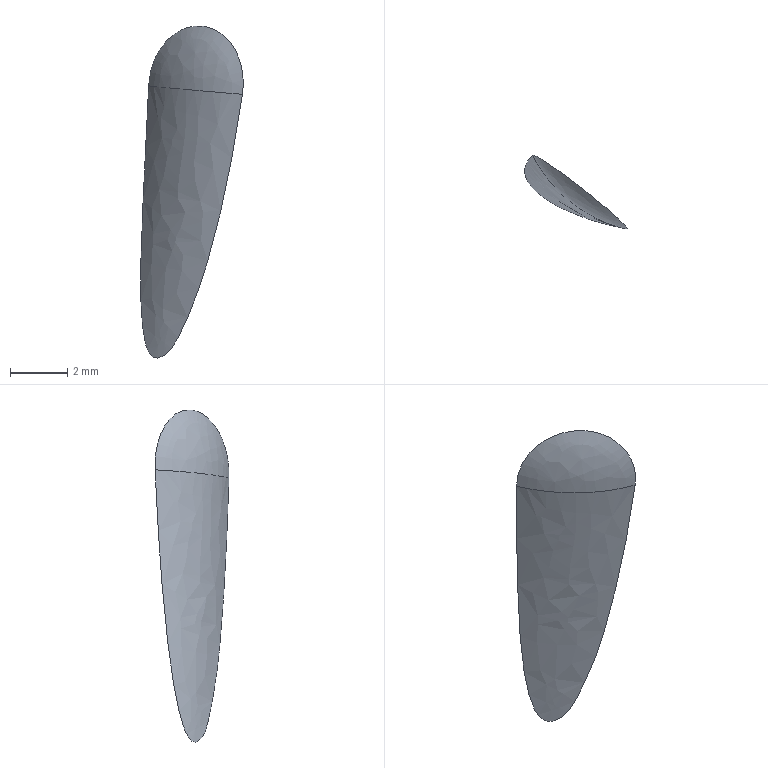Part | SolidWorks | features BaseBody 1 | 1 solid | 3 faces | box 3.595 x 2.597 x 11.647 mm | volume 8.243 mm3 | spline 3
STEP:
#1=CARTESIAN_POINT('',(82.6,89.025,-354.223));
#2=VERTEX_POINT('',#1);
#3=CARTESIAN_POINT('',(82.21,90.498,-344.695));
#4=VERTEX_POINT('',#3);
#5=CARTESIAN_POINT('',(82.6,89.025,-354.223));
#6=CARTESIAN_POINT('',(82.57,89.045,-354.233));
#7=CARTESIAN_POINT('',(82.541,89.067,-354.239));
#8=CARTESIAN_POINT('',(82.482,89.112,-354.242));
#9=CARTESIAN_POINT('',(82.452,89.136,-354.238));
#10=CARTESIAN_POINT('',(82.396,89.181,-354.222));
#11=CARTESIAN_POINT('',(82.356,89.215,-354.202));
#12=CARTESIAN_POINT('',(82.314,89.253,-354.167));
#13=CARTESIAN_POINT('',(82.294,89.272,-354.147));
#14=CARTESIAN_POINT('',(82.285,89.28,-354.137));
#15=CARTESIAN_POINT('',(82.28,89.286,-354.131));
#16=CARTESIAN_POINT('',(82.278,89.288,-354.128));
#17=CARTESIAN_POINT('',(82.246,89.319,-354.089));
#18=CARTESIAN_POINT('',(82.207,89.359,-354.027));
#19=CARTESIAN_POINT('',(82.167,89.405,-353.935));
#20=CARTESIAN_POINT('',(82.148,89.428,-353.885));
#21=CARTESIAN_POINT('',(82.14,89.437,-353.863));
#22=CARTESIAN_POINT('',(82.135,89.444,-353.848));
#23=CARTESIAN_POINT('',(82.132,89.447,-353.841));
#24=CARTESIAN_POINT('',(82.106,89.48,-353.76));
#25=CARTESIAN_POINT('',(82.085,89.51,-353.677));
#26=CARTESIAN_POINT('',(82.056,89.554,-353.538));
#27=CARTESIAN_POINT('',(82.043,89.576,-353.464));
#28=CARTESIAN_POINT('',(82.028,89.602,-353.372));
#29=CARTESIAN_POINT('',(82.021,89.615,-353.324));
#30=CARTESIAN_POINT('',(82.018,89.621,-353.303));
#31=CARTESIAN_POINT('',(82.016,89.624,-353.289));
#32=CARTESIAN_POINT('',(82.016,89.626,-353.284));
#33=CARTESIAN_POINT('',(81.977,89.702,-352.99));
#34=CARTESIAN_POINT('',(81.953,89.773,-352.649));
#35=CARTESIAN_POINT('',(81.935,89.875,-352.053));
#36=CARTESIAN_POINT('',(81.933,89.908,-351.84));
#37=CARTESIAN_POINT('',(81.933,89.957,-351.5));
#38=CARTESIAN_POINT('',(81.934,89.981,-351.325));
#39=CARTESIAN_POINT('',(81.936,90.008,-351.111));
#40=CARTESIAN_POINT('',(81.938,90.022,-351.002));
#41=CARTESIAN_POINT('',(81.939,90.029,-350.947));
#42=CARTESIAN_POINT('',(81.94,90.032,-350.919));
#43=CARTESIAN_POINT('',(81.94,90.034,-350.907));
#44=CARTESIAN_POINT('',(81.94,90.035,-350.899));
#45=CARTESIAN_POINT('',(81.94,90.035,-350.898));
#46=CARTESIAN_POINT('',(81.971,90.229,-349.305));
#47=CARTESIAN_POINT('',(82.097,90.382,-347.242));
#48=CARTESIAN_POINT('',(82.21,90.498,-344.695));
#49=B_SPLINE_CURVE_WITH_KNOTS('',3,(#5,#6,#7,#8,#9,#10,#11,#12,#13,#14,#15,#16,#17,#18,#19,#20,#21,#22,#23,#24,#25,#26,#27,#28,#29,#30,#31,#32,#33,#34,#35,#36,#37,#38,#39,#40,#41,#42,#43,#44,#45,#46,#47,#48),.UNSPECIFIED.,.F.,.F.,(4,2,2,1,1,1,2,2,1,1,1,2,2,2,1,1,1,2,2,2,2,1,1,1,1,1,2,2,4),(0.,0.0625,0.125,0.1875,0.2187,0.2344,0.2422,0.25,0.3125,0.3437,0.3594,0.3672,0.375,0.4375,0.4687,0.4844,0.4922,0.4961,0.5,0.625,0.6875,0.7187,0.7344,0.7422,0.7461,0.748,0.749,0.75,1.),.UNSPECIFIED.);
#50=EDGE_CURVE('',#2,#4,#49,.T.);
#51=ORIENTED_EDGE('',*,*,#50,.T.);
#52=CARTESIAN_POINT('',(85.499,87.906,-344.992));
#53=VERTEX_POINT('',#52);
#54=CARTESIAN_POINT('',(82.21,90.498,-344.695));
#55=CARTESIAN_POINT('',(82.217,90.504,-344.55));
#56=CARTESIAN_POINT('',(82.235,90.502,-344.408));
#57=CARTESIAN_POINT('',(82.293,90.48,-344.129));
#58=CARTESIAN_POINT('',(82.334,90.459,-343.99));
#59=CARTESIAN_POINT('',(82.436,90.402,-343.727));
#60=CARTESIAN_POINT('',(82.496,90.366,-343.603));
#61=CARTESIAN_POINT('',(82.637,90.276,-343.368));
#62=CARTESIAN_POINT('',(82.717,90.223,-343.258));
#63=CARTESIAN_POINT('',(82.977,90.047,-342.965));
#64=CARTESIAN_POINT('',(83.182,89.9,-342.812));
#65=CARTESIAN_POINT('',(83.507,89.66,-342.668));
#66=CARTESIAN_POINT('',(83.621,89.575,-342.633));
#67=CARTESIAN_POINT('',(83.847,89.402,-342.594));
#68=CARTESIAN_POINT('',(83.96,89.314,-342.589));
#69=CARTESIAN_POINT('',(84.186,89.136,-342.609));
#70=CARTESIAN_POINT('',(84.298,89.046,-342.635));
#71=CARTESIAN_POINT('',(84.511,88.873,-342.713));
#72=CARTESIAN_POINT('',(84.615,88.787,-342.766));
#73=CARTESIAN_POINT('',(84.811,88.622,-342.9));
#74=CARTESIAN_POINT('',(84.902,88.544,-342.98));
#75=CARTESIAN_POINT('',(85.068,88.398,-343.161));
#76=CARTESIAN_POINT('',(85.145,88.329,-343.265));
#77=CARTESIAN_POINT('',(85.277,88.206,-343.488));
#78=CARTESIAN_POINT('',(85.333,88.152,-343.608));
#79=CARTESIAN_POINT('',(85.426,88.057,-343.864));
#80=CARTESIAN_POINT('',(85.462,88.017,-344.));
#81=CARTESIAN_POINT('',(85.536,87.925,-344.412));
#82=CARTESIAN_POINT('',(85.541,87.897,-344.705));
#83=CARTESIAN_POINT('',(85.499,87.906,-344.992));
#84=B_SPLINE_CURVE_WITH_KNOTS('',3,(#54,#55,#56,#57,#58,#59,#60,#61,#62,#63,#64,#65,#66,#67,#68,#69,#70,#71,#72,#73,#74,#75,#76,#77,#78,#79,#80,#81,#82,#83),.UNSPECIFIED.,.F.,.F.,(4,2,2,2,2,2,2,2,2,2,2,2,2,2,4),(0.,0.0004292,0.0008585,0.001288,0.001717,0.002575,0.003005,0.003434,0.003863,0.004292,0.004722,0.005151,0.00558,0.006009,0.006868),.UNSPECIFIED.);
#85=EDGE_CURVE('',#4,#53,#84,.T.);
#86=ORIENTED_EDGE('',*,*,#85,.T.);
#87=CARTESIAN_POINT('',(83.582,88.495,-352.819));
#88=VERTEX_POINT('',#87);
#89=CARTESIAN_POINT('',(85.499,87.906,-344.992));
#90=CARTESIAN_POINT('',(85.364,87.934,-345.952));
#91=CARTESIAN_POINT('',(85.208,87.97,-346.869));
#92=CARTESIAN_POINT('',(85.012,88.019,-347.849));
#93=CARTESIAN_POINT('',(84.987,88.026,-347.971));
#94=CARTESIAN_POINT('',(84.961,88.032,-348.092));
#95=CARTESIAN_POINT('',(84.956,88.034,-348.119));
#96=CARTESIAN_POINT('',(84.954,88.034,-348.129));
#97=CARTESIAN_POINT('',(84.947,88.036,-348.163));
#98=CARTESIAN_POINT('',(84.932,88.04,-348.231));
#99=CARTESIAN_POINT('',(84.88,88.054,-348.478));
#100=CARTESIAN_POINT('',(84.831,88.066,-348.696));
#101=CARTESIAN_POINT('',(84.715,88.098,-349.208));
#102=CARTESIAN_POINT('',(84.636,88.12,-349.532));
#103=CARTESIAN_POINT('',(84.518,88.154,-349.995));
#104=CARTESIAN_POINT('',(84.478,88.166,-350.145));
#105=CARTESIAN_POINT('',(84.419,88.184,-350.365));
#106=CARTESIAN_POINT('',(84.4,88.19,-350.432));
#107=CARTESIAN_POINT('',(84.364,88.201,-350.564));
#108=CARTESIAN_POINT('',(84.272,88.23,-350.89));
#109=CARTESIAN_POINT('',(84.182,88.259,-351.186));
#110=CARTESIAN_POINT('',(84.094,88.289,-351.458));
#111=CARTESIAN_POINT('',(84.076,88.296,-351.512));
#112=CARTESIAN_POINT('',(84.05,88.305,-351.59));
#113=CARTESIAN_POINT('',(84.04,88.309,-351.621));
#114=CARTESIAN_POINT('',(84.019,88.316,-351.682));
#115=CARTESIAN_POINT('',(83.968,88.334,-351.832));
#116=CARTESIAN_POINT('',(83.907,88.357,-352.001));
#117=CARTESIAN_POINT('',(83.857,88.376,-352.134));
#118=CARTESIAN_POINT('',(83.838,88.384,-352.187));
#119=CARTESIAN_POINT('',(83.826,88.389,-352.218));
#120=CARTESIAN_POINT('',(83.792,88.402,-352.306));
#121=CARTESIAN_POINT('',(83.72,88.431,-352.488));
#122=CARTESIAN_POINT('',(83.638,88.465,-352.683));
#123=CARTESIAN_POINT('',(83.582,88.495,-352.819));
#124=B_SPLINE_CURVE_WITH_KNOTS('',3,(#89,#90,#91,#92,#93,#94,#95,#96,#97,#98,#99,#100,#101,#102,#103,#104,#105,#106,#107,#108,#109,#110,#111,#112,#113,#114,#115,#116,#117,#118,#119,#120,#121,#122,#123),.UNSPECIFIED.,.F.,.F.,(4,2,1,2,2,1,1,2,2,2,2,1,2,2,2,1,1,2,2,1,4),(0.,0.25,0.2812,0.2852,0.2891,0.2969,0.3125,0.375,0.5,0.5625,0.5937,0.625,0.75,0.7812,0.7969,0.8125,0.875,0.8906,0.9062,0.9375,1.),.UNSPECIFIED.);
#125=EDGE_CURVE('',#53,#88,#124,.T.);
#126=ORIENTED_EDGE('',*,*,#125,.T.);
#127=CARTESIAN_POINT('',(83.582,88.495,-352.819));
#128=CARTESIAN_POINT('',(83.486,88.53,-353.036));
#129=CARTESIAN_POINT('',(83.4,88.567,-353.222));
#130=CARTESIAN_POINT('',(83.283,88.62,-353.458));
#131=CARTESIAN_POINT('',(83.228,88.646,-353.566));
#132=CARTESIAN_POINT('',(83.17,88.674,-353.671));
#133=CARTESIAN_POINT('',(83.142,88.688,-353.719));
#134=CARTESIAN_POINT('',(83.13,88.693,-353.739));
#135=CARTESIAN_POINT('',(83.123,88.697,-353.752));
#136=CARTESIAN_POINT('',(83.12,88.699,-353.756));
#137=CARTESIAN_POINT('',(83.038,88.74,-353.89));
#138=CARTESIAN_POINT('',(82.959,88.785,-353.988));
#139=CARTESIAN_POINT('',(82.791,88.891,-354.139));
#140=CARTESIAN_POINT('',(82.699,88.953,-354.192));
#141=CARTESIAN_POINT('',(82.6,89.025,-354.223));
#142=B_SPLINE_CURVE_WITH_KNOTS('',3,(#127,#128,#129,#130,#131,#132,#133,#134,#135,#136,#137,#138,#139,#140,#141),.UNSPECIFIED.,.F.,.F.,(4,2,1,1,1,2,2,2,4),(0.,0.25,0.375,0.4375,0.4687,0.4844,0.5,0.75,1.),.UNSPECIFIED.);
#143=EDGE_CURVE('',#88,#2,#142,.T.);
#144=ORIENTED_EDGE('',*,*,#143,.T.);
#145=EDGE_LOOP('',(#51,#86,#126,#144));
#146=FACE_OUTER_BOUND('',#145,.T.);
#147=CARTESIAN_POINT('',(80.597,90.552,-354.062));
#148=CARTESIAN_POINT('',(81.739,89.68,-354.318));
#149=CARTESIAN_POINT('',(82.858,88.78,-354.569));
#150=CARTESIAN_POINT('',(83.956,87.851,-354.815));
#151=CARTESIAN_POINT('',(81.471,90.552,-350.165));
#152=CARTESIAN_POINT('',(82.624,89.68,-350.366));
#153=CARTESIAN_POINT('',(83.756,88.78,-350.563));
#154=CARTESIAN_POINT('',(84.866,87.851,-350.756));
#155=CARTESIAN_POINT('',(82.06,90.552,-346.215));
#156=CARTESIAN_POINT('',(83.222,89.68,-346.36));
#157=CARTESIAN_POINT('',(84.362,88.78,-346.502));
#158=CARTESIAN_POINT('',(85.479,87.851,-346.641));
#159=CARTESIAN_POINT('',(82.361,90.552,-342.233));
#160=CARTESIAN_POINT('',(83.527,89.68,-342.321));
#161=CARTESIAN_POINT('',(84.671,88.78,-342.408));
#162=CARTESIAN_POINT('',(85.793,87.851,-342.493));
#163=(BOUNDED_SURFACE()B_SPLINE_SURFACE(3,3,((#147,#148,#149,#150),(#151,#152,#153,#154),(#155,#156,#157,#158),(#159,#160,#161,#162)),.UNSPECIFIED.,.F.,.F.,.T.)B_SPLINE_SURFACE_WITH_KNOTS((4,4),(4,4),(0.,1.),(0.,1.),.UNSPECIFIED.)GEOMETRIC_REPRESENTATION_ITEM()RATIONAL_B_SPLINE_SURFACE(((1.001,1.001,1.001,1.001),(0.9997,0.9995,0.9995,0.9997),(0.9997,0.9995,0.9995,0.9997),(1.001,1.001,1.001,1.001)))REPRESENTATION_ITEM('')SURFACE());
#164=ADVANCED_FACE('',(#146),#163,.T.);
#165=ORIENTED_EDGE('',*,*,#85,.F.);
#166=CARTESIAN_POINT('',(82.21,90.498,-344.695));
#167=CARTESIAN_POINT('',(82.301,90.32,-344.705));
#168=CARTESIAN_POINT('',(82.399,90.153,-344.716));
#169=CARTESIAN_POINT('',(82.552,89.922,-344.731));
#170=CARTESIAN_POINT('',(82.605,89.848,-344.737));
#171=CARTESIAN_POINT('',(82.684,89.741,-344.745));
#172=CARTESIAN_POINT('',(82.724,89.689,-344.749));
#173=CARTESIAN_POINT('',(82.771,89.63,-344.753));
#174=CARTESIAN_POINT('',(82.791,89.605,-344.755));
#175=CARTESIAN_POINT('',(82.805,89.589,-344.756));
#176=CARTESIAN_POINT('',(82.81,89.582,-344.757));
#177=CARTESIAN_POINT('',(82.944,89.42,-344.77));
#178=CARTESIAN_POINT('',(83.075,89.281,-344.783));
#179=CARTESIAN_POINT('',(83.275,89.09,-344.801));
#180=CARTESIAN_POINT('',(83.342,89.029,-344.807));
#181=CARTESIAN_POINT('',(83.444,88.942,-344.817));
#182=CARTESIAN_POINT('',(83.495,88.899,-344.821));
#183=CARTESIAN_POINT('',(83.554,88.852,-344.827));
#184=CARTESIAN_POINT('',(83.58,88.832,-344.829));
#185=CARTESIAN_POINT('',(83.597,88.818,-344.83));
#186=CARTESIAN_POINT('',(83.604,88.812,-344.831));
#187=CARTESIAN_POINT('',(83.918,88.57,-344.859));
#188=CARTESIAN_POINT('',(84.232,88.384,-344.887));
#189=CARTESIAN_POINT('',(84.862,88.091,-344.94));
#190=CARTESIAN_POINT('',(85.178,87.983,-344.966));
#191=CARTESIAN_POINT('',(85.499,87.906,-344.992));
#192=B_SPLINE_CURVE_WITH_KNOTS('',3,(#166,#167,#168,#169,#170,#171,#172,#173,#174,#175,#176,#177,#178,#179,#180,#181,#182,#183,#184,#185,#186,#187,#188,#189,#190,#191),.UNSPECIFIED.,.F.,.F.,(4,2,2,1,1,2,2,2,2,1,1,2,2,2,4),(0.,0.125,0.1875,0.2187,0.2344,0.2422,0.25,0.375,0.4375,0.4687,0.4844,0.4922,0.5,0.75,1.),.UNSPECIFIED.);
#193=EDGE_CURVE('',#4,#53,#192,.T.);
#194=ORIENTED_EDGE('',*,*,#193,.T.);
#195=EDGE_LOOP('',(#165,#194));
#196=FACE_OUTER_BOUND('',#195,.T.);
#197=CARTESIAN_POINT('',(84.713,89.114,-342.197));
#198=CARTESIAN_POINT('',(84.708,88.608,-342.86));
#199=CARTESIAN_POINT('',(85.179,88.19,-343.408));
#200=CARTESIAN_POINT('',(85.958,88.009,-343.646));
#201=CARTESIAN_POINT('',(83.505,89.523,-342.5));
#202=CARTESIAN_POINT('',(83.497,88.702,-343.576));
#203=CARTESIAN_POINT('',(84.261,88.023,-344.465));
#204=CARTESIAN_POINT('',(85.526,87.729,-344.851));
#205=CARTESIAN_POINT('',(82.575,90.26,-343.056));
#206=CARTESIAN_POINT('',(82.565,89.196,-344.45));
#207=CARTESIAN_POINT('',(83.555,88.318,-345.602));
#208=CARTESIAN_POINT('',(85.192,87.937,-346.101));
#209=CARTESIAN_POINT('',(82.058,91.22,-343.784));
#210=CARTESIAN_POINT('',(82.047,90.021,-345.355));
#211=CARTESIAN_POINT('',(83.162,89.031,-346.652));
#212=CARTESIAN_POINT('',(85.007,88.602,-347.215));
#213=(BOUNDED_SURFACE()B_SPLINE_SURFACE(3,3,((#197,#198,#199,#200),(#201,#202,#203,#204),(#205,#206,#207,#208),(#209,#210,#211,#212)),.UNSPECIFIED.,.F.,.F.,.T.)B_SPLINE_SURFACE_WITH_KNOTS((4,4),(4,4),(0.,1.),(0.,1.),.UNSPECIFIED.)GEOMETRIC_REPRESENTATION_ITEM()RATIONAL_B_SPLINE_SURFACE(((1.,0.8817,0.8817,1.),(0.9516,0.839,0.839,0.9516),(0.9516,0.839,0.839,0.9516),(1.,0.8817,0.8817,1.)))REPRESENTATION_ITEM('')SURFACE());
#214=ADVANCED_FACE('',(#196),#213,.T.);
#215=ORIENTED_EDGE('',*,*,#125,.F.);
#216=ORIENTED_EDGE('',*,*,#193,.F.);
#217=ORIENTED_EDGE('',*,*,#50,.F.);
#218=ORIENTED_EDGE('',*,*,#143,.F.);
#219=EDGE_LOOP('',(#215,#216,#217,#218));
#220=FACE_OUTER_BOUND('',#219,.T.);
#221=CARTESIAN_POINT('',(81.013,90.974,-354.007));
#222=CARTESIAN_POINT('',(81.6,89.671,-354.168));
#223=CARTESIAN_POINT('',(82.653,88.747,-354.385));
#224=CARTESIAN_POINT('',(83.96,88.321,-354.617));
#225=CARTESIAN_POINT('',(81.551,90.748,-350.868));
#226=CARTESIAN_POINT('',(82.185,89.405,-350.993));
#227=CARTESIAN_POINT('',(83.306,88.479,-351.183));
#228=CARTESIAN_POINT('',(84.677,88.093,-351.397));
#229=CARTESIAN_POINT('',(81.944,90.617,-347.741));
#230=CARTESIAN_POINT('',(82.611,89.247,-347.841));
#231=CARTESIAN_POINT('',(83.786,88.323,-347.991));
#232=CARTESIAN_POINT('',(85.208,87.97,-348.157));
#233=CARTESIAN_POINT('',(82.198,90.535,-344.6));
#234=CARTESIAN_POINT('',(82.888,89.147,-344.676));
#235=CARTESIAN_POINT('',(84.098,88.225,-344.784));
#236=CARTESIAN_POINT('',(85.552,87.894,-344.9));
#237=(BOUNDED_SURFACE()B_SPLINE_SURFACE(3,3,((#221,#222,#223,#224),(#225,#226,#227,#228),(#229,#230,#231,#232),(#233,#234,#235,#236)),.UNSPECIFIED.,.F.,.F.,.F.)B_SPLINE_SURFACE_WITH_KNOTS((4,4),(4,4),(-0.003738,1.01),(-0.003424,1.004),.UNSPECIFIED.)GEOMETRIC_REPRESENTATION_ITEM()RATIONAL_B_SPLINE_SURFACE(((0.9117,0.8861,0.9144,0.9968),(0.9064,0.8791,0.9092,0.9966),(0.9022,0.8738,0.9052,0.9965),(0.8995,0.8703,0.9026,0.9964)))REPRESENTATION_ITEM('')SURFACE());
#238=ADVANCED_FACE('',(#220),#237,.F.);
#239=CLOSED_SHELL('',(#164,#214,#238));
#240=MANIFOLD_SOLID_BREP('',#239);
#241=CARTESIAN_POINT('',(0.,0.,0.));
#242=DIRECTION('',(0.,0.,1.));
#243=DIRECTION('',(1.,0.,0.));
#244=AXIS2_PLACEMENT_3D('',#241,#242,#243);
#245=(LENGTH_UNIT()NAMED_UNIT(*)SI_UNIT(.MILLI.,.METRE.));
#246=UNCERTAINTY_MEASURE_WITH_UNIT(LENGTH_MEASURE(0.00001),#245,'','');
#247=(NAMED_UNIT(*)PLANE_ANGLE_UNIT()SI_UNIT($,.RADIAN.));
#248=(NAMED_UNIT(*)SI_UNIT($,.STERADIAN.)SOLID_ANGLE_UNIT());
#249=(GEOMETRIC_REPRESENTATION_CONTEXT(3)GLOBAL_UNCERTAINTY_ASSIGNED_CONTEXT((#246))GLOBAL_UNIT_ASSIGNED_CONTEXT((#245,#247,#248))REPRESENTATION_CONTEXT('',''));
#250=ADVANCED_BREP_SHAPE_REPRESENTATION('',(#240,#244),#249);